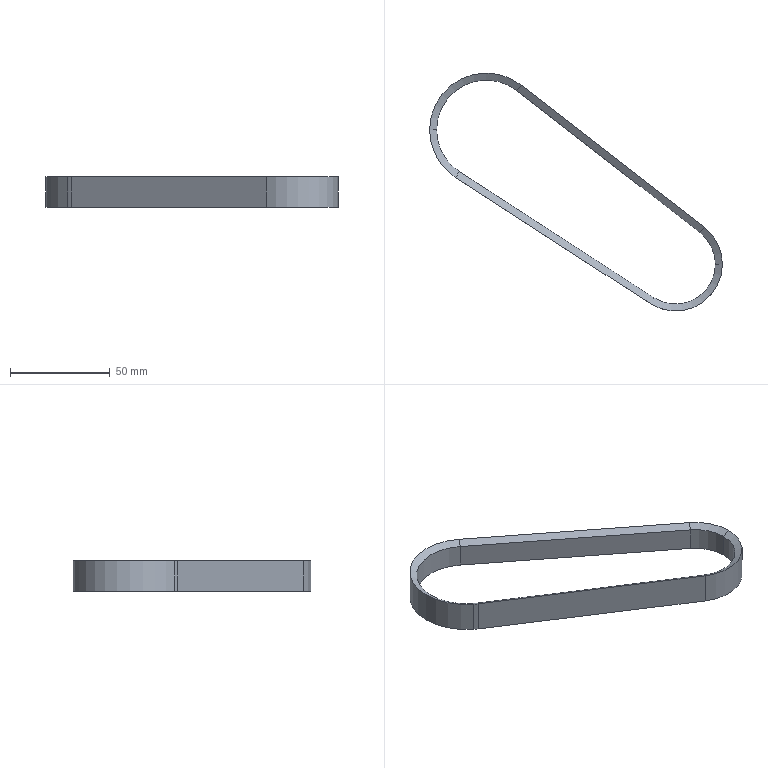Part | SolidWorks | features BaseBody 1 | 1 solid | 22 faces | box 147 x 119.5 x 15.423 mm | volume 18116 mm3 | cone 8 | plane 8 | cylinder 6 | commonest cylinder face diameters 40 x2 57 x2 47 x1 50 x1
STEP:
#1=CARTESIAN_POINT('',(-10.874,-16.786,2.021));
#2=VERTEX_POINT('',#1);
#3=CARTESIAN_POINT('',(20.,0.,2.021));
#4=VERTEX_POINT('',#3);
#5=CARTESIAN_POINT('',(0.,0.,2.021));
#6=DIRECTION('',(0.,0.,1.));
#7=DIRECTION('',(1.,0.,0.));
#8=AXIS2_PLACEMENT_3D('',#5,#6,#7);
#9=CIRCLE('',#8,20.);
#10=EDGE_CURVE('',#2,#4,#9,.T.);
#11=ORIENTED_EDGE('',*,*,#10,.T.);
#12=CARTESIAN_POINT('',(23.5,0.,0.));
#13=VERTEX_POINT('',#12);
#14=CARTESIAN_POINT('',(21.75,0.,1.01));
#15=DIRECTION('',(0.866,0.,-0.5001));
#16=VECTOR('',#15,1000.);
#17=LINE('',#14,#16);
#18=EDGE_CURVE('',#4,#13,#17,.T.);
#19=ORIENTED_EDGE('',*,*,#18,.T.);
#20=CARTESIAN_POINT('',(-12.777,-19.723,0.));
#21=VERTEX_POINT('',#20);
#22=CARTESIAN_POINT('',(0.,0.,0.));
#23=DIRECTION('',(0.,0.,-1.));
#24=DIRECTION('',(0.5437,0.8393,0.));
#25=AXIS2_PLACEMENT_3D('',#22,#23,#24);
#26=CIRCLE('',#25,23.5);
#27=EDGE_CURVE('',#13,#21,#26,.T.);
#28=ORIENTED_EDGE('',*,*,#27,.T.);
#29=CARTESIAN_POINT('',(-10.874,-16.786,2.021));
#30=DIRECTION('',(-0.4708,-0.7268,-0.5001));
#31=VECTOR('',#30,1000.);
#32=LINE('',#29,#31);
#33=EDGE_CURVE('',#2,#21,#32,.T.);
#34=ORIENTED_EDGE('',*,*,#33,.F.);
#35=EDGE_LOOP('',(#11,#19,#28,#34));
#36=FACE_OUTER_BOUND('',#35,.T.);
#37=CARTESIAN_POINT('',(0.,0.,1.01));
#38=DIRECTION('',(0.,0.,-1.));
#39=DIRECTION('',(1.,0.,0.));
#40=AXIS2_PLACEMENT_3D('',#37,#38,#39);
#41=CONICAL_SURFACE('',#40,21.75,1.047);
#42=ADVANCED_FACE('',(#36),#41,.F.);
#43=CARTESIAN_POINT('',(-79.659,87.239,2.021));
#44=VERTEX_POINT('',#43);
#45=CARTESIAN_POINT('',(-120.,67.5,2.021));
#46=VERTEX_POINT('',#45);
#47=CARTESIAN_POINT('',(-95.,67.5,2.021));
#48=DIRECTION('',(0.,0.,1.));
#49=DIRECTION('',(-1.,0.,0.));
#50=AXIS2_PLACEMENT_3D('',#47,#48,#49);
#51=CIRCLE('',#50,25.);
#52=EDGE_CURVE('',#44,#46,#51,.T.);
#53=ORIENTED_EDGE('',*,*,#52,.T.);
#54=CARTESIAN_POINT('',(-123.5,67.5,0.));
#55=VERTEX_POINT('',#54);
#56=CARTESIAN_POINT('',(-121.75,67.5,1.01));
#57=DIRECTION('',(-0.866,0.,-0.5001));
#58=VECTOR('',#57,1000.);
#59=LINE('',#56,#58);
#60=EDGE_CURVE('',#46,#55,#59,.T.);
#61=ORIENTED_EDGE('',*,*,#60,.T.);
#62=CARTESIAN_POINT('',(-77.511,90.003,0.));
#63=VERTEX_POINT('',#62);
#64=CARTESIAN_POINT('',(-95.,67.5,0.));
#65=DIRECTION('',(0.,0.,-1.));
#66=DIRECTION('',(-0.6136,-0.7896,0.));
#67=AXIS2_PLACEMENT_3D('',#64,#65,#66);
#68=CIRCLE('',#67,28.5);
#69=EDGE_CURVE('',#55,#63,#68,.T.);
#70=ORIENTED_EDGE('',*,*,#69,.T.);
#71=CARTESIAN_POINT('',(-79.659,87.239,2.021));
#72=DIRECTION('',(0.5314,0.6838,-0.5001));
#73=VECTOR('',#72,1000.);
#74=LINE('',#71,#73);
#75=EDGE_CURVE('',#44,#63,#74,.T.);
#76=ORIENTED_EDGE('',*,*,#75,.F.);
#77=EDGE_LOOP('',(#53,#61,#70,#76));
#78=FACE_OUTER_BOUND('',#77,.T.);
#79=CARTESIAN_POINT('',(-95.,67.5,1.01));
#80=DIRECTION('',(0.,0.,-1.));
#81=DIRECTION('',(-1.,0.,0.));
#82=AXIS2_PLACEMENT_3D('',#79,#80,#81);
#83=CONICAL_SURFACE('',#82,26.75,1.047);
#84=ADVANCED_FACE('',(#78),#83,.F.);
#85=CARTESIAN_POINT('',(20.,0.,13.402));
#86=VERTEX_POINT('',#85);
#87=CARTESIAN_POINT('',(-10.874,-16.786,13.402));
#88=VERTEX_POINT('',#87);
#89=CARTESIAN_POINT('',(0.,0.,13.402));
#90=DIRECTION('',(0.,0.,-1.));
#91=DIRECTION('',(1.,0.,0.));
#92=AXIS2_PLACEMENT_3D('',#89,#90,#91);
#93=CIRCLE('',#92,20.);
#94=EDGE_CURVE('',#86,#88,#93,.T.);
#95=ORIENTED_EDGE('',*,*,#94,.F.);
#96=CARTESIAN_POINT('',(20.,0.,0.));
#97=DIRECTION('',(0.,0.,-1.));
#98=VECTOR('',#97,1000.);
#99=LINE('',#96,#98);
#100=EDGE_CURVE('',#86,#4,#99,.T.);
#101=ORIENTED_EDGE('',*,*,#100,.T.);
#102=ORIENTED_EDGE('',*,*,#10,.F.);
#103=CARTESIAN_POINT('',(-10.874,-16.786,0.));
#104=DIRECTION('',(0.,0.,-1.));
#105=VECTOR('',#104,1000.);
#106=LINE('',#103,#105);
#107=EDGE_CURVE('',#88,#2,#106,.T.);
#108=ORIENTED_EDGE('',*,*,#107,.F.);
#109=EDGE_LOOP('',(#95,#101,#102,#108));
#110=FACE_OUTER_BOUND('',#109,.T.);
#111=CARTESIAN_POINT('',(0.,0.,0.));
#112=DIRECTION('',(0.,0.,-1.));
#113=DIRECTION('',(1.,0.,0.));
#114=AXIS2_PLACEMENT_3D('',#111,#112,#113);
#115=CYLINDRICAL_SURFACE('',#114,20.);
#116=ADVANCED_FACE('',(#110),#115,.F.);
#117=CARTESIAN_POINT('',(12.273,15.792,13.402));
#118=VERTEX_POINT('',#117);
#119=CARTESIAN_POINT('',(0.,0.,13.402));
#120=DIRECTION('',(0.,0.,-1.));
#121=DIRECTION('',(1.,0.,0.));
#122=AXIS2_PLACEMENT_3D('',#119,#120,#121);
#123=CIRCLE('',#122,20.);
#124=EDGE_CURVE('',#118,#86,#123,.T.);
#125=ORIENTED_EDGE('',*,*,#124,.T.);
#126=CARTESIAN_POINT('',(23.5,0.,15.423));
#127=VERTEX_POINT('',#126);
#128=CARTESIAN_POINT('',(21.75,0.,14.412));
#129=DIRECTION('',(0.866,0.,0.5001));
#130=VECTOR('',#129,1000.);
#131=LINE('',#128,#130);
#132=EDGE_CURVE('',#86,#127,#131,.T.);
#133=ORIENTED_EDGE('',*,*,#132,.T.);
#134=CARTESIAN_POINT('',(14.421,18.555,15.423));
#135=VERTEX_POINT('',#134);
#136=CARTESIAN_POINT('',(0.,0.,15.423));
#137=DIRECTION('',(0.,0.,1.));
#138=DIRECTION('',(0.5437,0.8393,0.));
#139=AXIS2_PLACEMENT_3D('',#136,#137,#138);
#140=CIRCLE('',#139,23.5);
#141=EDGE_CURVE('',#127,#135,#140,.T.);
#142=ORIENTED_EDGE('',*,*,#141,.T.);
#143=CARTESIAN_POINT('',(14.421,18.555,15.423));
#144=DIRECTION('',(-0.5314,-0.6838,-0.5001));
#145=VECTOR('',#144,1000.);
#146=LINE('',#143,#145);
#147=EDGE_CURVE('',#135,#118,#146,.T.);
#148=ORIENTED_EDGE('',*,*,#147,.T.);
#149=EDGE_LOOP('',(#125,#133,#142,#148));
#150=FACE_OUTER_BOUND('',#149,.T.);
#151=CARTESIAN_POINT('',(0.,0.,14.412));
#152=DIRECTION('',(0.,0.,1.));
#153=DIRECTION('',(1.,0.,0.));
#154=AXIS2_PLACEMENT_3D('',#151,#152,#153);
#155=CONICAL_SURFACE('',#154,21.75,1.047);
#156=ADVANCED_FACE('',(#150),#155,.F.);
#157=CARTESIAN_POINT('',(-108.592,46.518,13.402));
#158=VERTEX_POINT('',#157);
#159=CARTESIAN_POINT('',(-120.,67.5,13.402));
#160=VERTEX_POINT('',#159);
#161=CARTESIAN_POINT('',(-95.,67.5,13.402));
#162=DIRECTION('',(0.,0.,-1.));
#163=DIRECTION('',(-1.,0.,0.));
#164=AXIS2_PLACEMENT_3D('',#161,#162,#163);
#165=CIRCLE('',#164,25.);
#166=EDGE_CURVE('',#158,#160,#165,.T.);
#167=ORIENTED_EDGE('',*,*,#166,.T.);
#168=CARTESIAN_POINT('',(-123.5,67.5,15.423));
#169=VERTEX_POINT('',#168);
#170=CARTESIAN_POINT('',(-121.75,67.5,14.412));
#171=DIRECTION('',(-0.866,0.,0.5001));
#172=VECTOR('',#171,1000.);
#173=LINE('',#170,#172);
#174=EDGE_CURVE('',#160,#169,#173,.T.);
#175=ORIENTED_EDGE('',*,*,#174,.T.);
#176=CARTESIAN_POINT('',(-112.489,44.997,15.423));
#177=VERTEX_POINT('',#176);
#178=CARTESIAN_POINT('',(-95.,67.5,15.423));
#179=DIRECTION('',(0.,0.,1.));
#180=DIRECTION('',(-0.6136,-0.7896,0.));
#181=AXIS2_PLACEMENT_3D('',#178,#179,#180);
#182=CIRCLE('',#181,28.5);
#183=EDGE_CURVE('',#169,#177,#182,.T.);
#184=ORIENTED_EDGE('',*,*,#183,.T.);
#185=CARTESIAN_POINT('',(-110.495,43.581,15.423));
#186=VERTEX_POINT('',#185);
#187=CARTESIAN_POINT('',(-95.,67.5,15.423));
#188=DIRECTION('',(0.,0.,1.));
#189=DIRECTION('',(-0.6136,-0.7896,0.));
#190=AXIS2_PLACEMENT_3D('',#187,#188,#189);
#191=CIRCLE('',#190,28.5);
#192=EDGE_CURVE('',#177,#186,#191,.T.);
#193=ORIENTED_EDGE('',*,*,#192,.T.);
#194=CARTESIAN_POINT('',(-108.592,46.518,13.402));
#195=DIRECTION('',(-0.4708,-0.7268,0.5001));
#196=VECTOR('',#195,1000.);
#197=LINE('',#194,#196);
#198=EDGE_CURVE('',#158,#186,#197,.T.);
#199=ORIENTED_EDGE('',*,*,#198,.F.);
#200=EDGE_LOOP('',(#167,#175,#184,#193,#199));
#201=FACE_OUTER_BOUND('',#200,.T.);
#202=CARTESIAN_POINT('',(-95.,67.5,14.412));
#203=DIRECTION('',(0.,0.,1.));
#204=DIRECTION('',(-1.,0.,0.));
#205=AXIS2_PLACEMENT_3D('',#202,#203,#204);
#206=CONICAL_SURFACE('',#205,26.75,1.047);
#207=ADVANCED_FACE('',(#201),#206,.F.);
#208=ORIENTED_EDGE('',*,*,#192,.F.);
#209=CARTESIAN_POINT('',(-112.489,44.997,0.));
#210=VERTEX_POINT('',#209);
#211=CARTESIAN_POINT('',(-112.489,44.997,0.));
#212=DIRECTION('',(0.,0.,-1.));
#213=VECTOR('',#212,1000.);
#214=LINE('',#211,#213);
#215=EDGE_CURVE('',#177,#210,#214,.T.);
#216=ORIENTED_EDGE('',*,*,#215,.T.);
#217=CARTESIAN_POINT('',(-110.495,43.581,0.));
#218=VERTEX_POINT('',#217);
#219=CARTESIAN_POINT('',(-95.,67.5,0.));
#220=DIRECTION('',(0.,0.,-1.));
#221=DIRECTION('',(-0.6136,-0.7896,0.));
#222=AXIS2_PLACEMENT_3D('',#219,#220,#221);
#223=CIRCLE('',#222,28.5);
#224=EDGE_CURVE('',#218,#210,#223,.T.);
#225=ORIENTED_EDGE('',*,*,#224,.F.);
#226=CARTESIAN_POINT('',(-110.495,43.581,0.));
#227=DIRECTION('',(0.,0.,1.));
#228=VECTOR('',#227,1000.);
#229=LINE('',#226,#228);
#230=EDGE_CURVE('',#218,#186,#229,.T.);
#231=ORIENTED_EDGE('',*,*,#230,.T.);
#232=EDGE_LOOP('',(#208,#216,#225,#231));
#233=FACE_OUTER_BOUND('',#232,.T.);
#234=CARTESIAN_POINT('',(-95.,67.5,0.));
#235=DIRECTION('',(0.,0.,-1.));
#236=DIRECTION('',(-0.6136,-0.7896,0.));
#237=AXIS2_PLACEMENT_3D('',#234,#235,#236);
#238=CYLINDRICAL_SURFACE('',#237,28.5);
#239=ADVANCED_FACE('',(#233),#238,.T.);
#240=ORIENTED_EDGE('',*,*,#33,.T.);
#241=CARTESIAN_POINT('',(-12.777,-19.723,0.));
#242=DIRECTION('',(-0.8393,0.5437,0.));
#243=VECTOR('',#242,1000.);
#244=LINE('',#241,#243);
#245=EDGE_CURVE('',#21,#218,#244,.T.);
#246=ORIENTED_EDGE('',*,*,#245,.T.);
#247=CARTESIAN_POINT('',(-108.592,46.518,2.021));
#248=VERTEX_POINT('',#247);
#249=CARTESIAN_POINT('',(-110.495,43.581,0.));
#250=DIRECTION('',(0.4708,0.7268,0.5001));
#251=VECTOR('',#250,1000.);
#252=LINE('',#249,#251);
#253=EDGE_CURVE('',#218,#248,#252,.T.);
#254=ORIENTED_EDGE('',*,*,#253,.T.);
#255=CARTESIAN_POINT('',(-85.355,31.464,2.021));
#256=DIRECTION('',(0.8393,-0.5437,0.));
#257=VECTOR('',#256,1000.);
#258=LINE('',#255,#257);
#259=EDGE_CURVE('',#248,#2,#258,.T.);
#260=ORIENTED_EDGE('',*,*,#259,.T.);
#261=EDGE_LOOP('',(#240,#246,#254,#260));
#262=FACE_OUTER_BOUND('',#261,.T.);
#263=CARTESIAN_POINT('',(-86.306,29.996,1.01));
#264=DIRECTION('',(0.2719,0.4197,-0.866));
#265=DIRECTION('',(-0.9541,0.,-0.2995));
#266=AXIS2_PLACEMENT_3D('',#263,#264,#265);
#267=PLANE('',#266);
#268=ADVANCED_FACE('',(#262),#267,.T.);
#269=ORIENTED_EDGE('',*,*,#75,.T.);
#270=CARTESIAN_POINT('',(14.421,18.555,0.));
#271=VERTEX_POINT('',#270);
#272=CARTESIAN_POINT('',(-77.511,90.003,0.));
#273=DIRECTION('',(0.7896,-0.6136,0.));
#274=VECTOR('',#273,1000.);
#275=LINE('',#272,#274);
#276=EDGE_CURVE('',#63,#271,#275,.T.);
#277=ORIENTED_EDGE('',*,*,#276,.T.);
#278=CARTESIAN_POINT('',(12.273,15.792,2.021));
#279=VERTEX_POINT('',#278);
#280=CARTESIAN_POINT('',(12.273,15.792,2.021));
#281=DIRECTION('',(0.5314,0.6838,-0.5001));
#282=VECTOR('',#281,1000.);
#283=LINE('',#280,#282);
#284=EDGE_CURVE('',#279,#271,#283,.T.);
#285=ORIENTED_EDGE('',*,*,#284,.F.);
#286=CARTESIAN_POINT('',(-11.831,34.525,2.021));
#287=DIRECTION('',(-0.7896,0.6136,0.));
#288=VECTOR('',#287,1000.);
#289=LINE('',#286,#288);
#290=EDGE_CURVE('',#279,#44,#289,.T.);
#291=ORIENTED_EDGE('',*,*,#290,.T.);
#292=EDGE_LOOP('',(#269,#277,#285,#291));
#293=FACE_OUTER_BOUND('',#292,.T.);
#294=CARTESIAN_POINT('',(-10.758,35.907,1.01));
#295=DIRECTION('',(-0.3069,-0.3948,-0.866));
#296=DIRECTION('',(0.,-0.9099,0.4148));
#297=AXIS2_PLACEMENT_3D('',#294,#295,#296);
#298=PLANE('',#297);
#299=ADVANCED_FACE('',(#293),#298,.T.);
#300=ORIENTED_EDGE('',*,*,#259,.F.);
#301=CARTESIAN_POINT('',(-108.592,46.518,0.));
#302=DIRECTION('',(0.,0.,-1.));
#303=VECTOR('',#302,1000.);
#304=LINE('',#301,#303);
#305=EDGE_CURVE('',#158,#248,#304,.T.);
#306=ORIENTED_EDGE('',*,*,#305,.F.);
#307=CARTESIAN_POINT('',(-85.355,31.464,13.402));
#308=DIRECTION('',(-0.8393,0.5437,0.));
#309=VECTOR('',#308,1000.);
#310=LINE('',#307,#309);
#311=EDGE_CURVE('',#88,#158,#310,.T.);
#312=ORIENTED_EDGE('',*,*,#311,.F.);
#313=ORIENTED_EDGE('',*,*,#107,.T.);
#314=EDGE_LOOP('',(#300,#306,#312,#313));
#315=FACE_OUTER_BOUND('',#314,.T.);
#316=CARTESIAN_POINT('',(-108.592,46.518,0.));
#317=DIRECTION('',(-0.5437,-0.8393,0.));
#318=DIRECTION('',(-0.8393,0.5437,0.));
#319=AXIS2_PLACEMENT_3D('',#316,#317,#318);
#320=PLANE('',#319);
#321=ADVANCED_FACE('',(#315),#320,.F.);
#322=ORIENTED_EDGE('',*,*,#198,.T.);
#323=CARTESIAN_POINT('',(-12.777,-19.723,15.423));
#324=VERTEX_POINT('',#323);
#325=CARTESIAN_POINT('',(-12.777,-19.723,15.423));
#326=DIRECTION('',(0.8393,-0.5437,0.));
#327=VECTOR('',#326,1000.);
#328=LINE('',#325,#327);
#329=EDGE_CURVE('',#186,#324,#328,.T.);
#330=ORIENTED_EDGE('',*,*,#329,.T.);
#331=CARTESIAN_POINT('',(-10.874,-16.786,13.402));
#332=DIRECTION('',(-0.4708,-0.7268,0.5001));
#333=VECTOR('',#332,1000.);
#334=LINE('',#331,#333);
#335=EDGE_CURVE('',#88,#324,#334,.T.);
#336=ORIENTED_EDGE('',*,*,#335,.F.);
#337=ORIENTED_EDGE('',*,*,#311,.T.);
#338=EDGE_LOOP('',(#322,#330,#336,#337));
#339=FACE_OUTER_BOUND('',#338,.T.);
#340=CARTESIAN_POINT('',(-86.306,29.996,14.412));
#341=DIRECTION('',(0.2719,0.4197,0.866));
#342=DIRECTION('',(0.8393,-0.5437,0.));
#343=AXIS2_PLACEMENT_3D('',#340,#341,#342);
#344=PLANE('',#343);
#345=ADVANCED_FACE('',(#339),#344,.T.);
#346=ORIENTED_EDGE('',*,*,#147,.F.);
#347=CARTESIAN_POINT('',(-77.511,90.003,15.423));
#348=VERTEX_POINT('',#347);
#349=CARTESIAN_POINT('',(-77.511,90.003,15.423));
#350=DIRECTION('',(-0.7896,0.6136,0.));
#351=VECTOR('',#350,1000.);
#352=LINE('',#349,#351);
#353=EDGE_CURVE('',#135,#348,#352,.T.);
#354=ORIENTED_EDGE('',*,*,#353,.T.);
#355=CARTESIAN_POINT('',(-79.659,87.239,13.402));
#356=VERTEX_POINT('',#355);
#357=CARTESIAN_POINT('',(-79.659,87.239,13.402));
#358=DIRECTION('',(0.5314,0.6838,0.5001));
#359=VECTOR('',#358,1000.);
#360=LINE('',#357,#359);
#361=EDGE_CURVE('',#356,#348,#360,.T.);
#362=ORIENTED_EDGE('',*,*,#361,.F.);
#363=CARTESIAN_POINT('',(-11.831,34.525,13.402));
#364=DIRECTION('',(0.7896,-0.6136,0.));
#365=VECTOR('',#364,1000.);
#366=LINE('',#363,#365);
#367=EDGE_CURVE('',#356,#118,#366,.T.);
#368=ORIENTED_EDGE('',*,*,#367,.T.);
#369=EDGE_LOOP('',(#346,#354,#362,#368));
#370=FACE_OUTER_BOUND('',#369,.T.);
#371=CARTESIAN_POINT('',(-10.758,35.907,14.412));
#372=DIRECTION('',(-0.3069,-0.3948,0.866));
#373=DIRECTION('',(-0.7896,0.6136,0.));
#374=AXIS2_PLACEMENT_3D('',#371,#372,#373);
#375=PLANE('',#374);
#376=ADVANCED_FACE('',(#370),#375,.T.);
#377=ORIENTED_EDGE('',*,*,#290,.F.);
#378=CARTESIAN_POINT('',(12.273,15.792,0.));
#379=DIRECTION('',(0.,0.,-1.));
#380=VECTOR('',#379,1000.);
#381=LINE('',#378,#380);
#382=EDGE_CURVE('',#118,#279,#381,.T.);
#383=ORIENTED_EDGE('',*,*,#382,.F.);
#384=ORIENTED_EDGE('',*,*,#367,.F.);
#385=CARTESIAN_POINT('',(-79.659,87.239,0.));
#386=DIRECTION('',(0.,0.,-1.));
#387=VECTOR('',#386,1000.);
#388=LINE('',#385,#387);
#389=EDGE_CURVE('',#356,#44,#388,.T.);
#390=ORIENTED_EDGE('',*,*,#389,.T.);
#391=EDGE_LOOP('',(#377,#383,#384,#390));
#392=FACE_OUTER_BOUND('',#391,.T.);
#393=CARTESIAN_POINT('',(12.273,15.792,0.));
#394=DIRECTION('',(0.6136,0.7896,0.));
#395=DIRECTION('',(0.,0.,-1.));
#396=AXIS2_PLACEMENT_3D('',#393,#394,#395);
#397=PLANE('',#396);
#398=ADVANCED_FACE('',(#392),#397,.F.);
#399=ORIENTED_EDGE('',*,*,#52,.F.);
#400=ORIENTED_EDGE('',*,*,#389,.F.);
#401=CARTESIAN_POINT('',(-95.,67.5,13.402));
#402=DIRECTION('',(0.,0.,-1.));
#403=DIRECTION('',(-1.,0.,0.));
#404=AXIS2_PLACEMENT_3D('',#401,#402,#403);
#405=CIRCLE('',#404,25.);
#406=EDGE_CURVE('',#160,#356,#405,.T.);
#407=ORIENTED_EDGE('',*,*,#406,.F.);
#408=ORIENTED_EDGE('',*,*,#166,.F.);
#409=ORIENTED_EDGE('',*,*,#305,.T.);
#410=CARTESIAN_POINT('',(-95.,67.5,2.021));
#411=DIRECTION('',(0.,0.,1.));
#412=DIRECTION('',(-1.,0.,0.));
#413=AXIS2_PLACEMENT_3D('',#410,#411,#412);
#414=CIRCLE('',#413,25.);
#415=EDGE_CURVE('',#46,#248,#414,.T.);
#416=ORIENTED_EDGE('',*,*,#415,.F.);
#417=EDGE_LOOP('',(#399,#400,#407,#408,#409,#416));
#418=FACE_OUTER_BOUND('',#417,.T.);
#419=CARTESIAN_POINT('',(-95.,67.5,0.));
#420=DIRECTION('',(0.,0.,-1.));
#421=DIRECTION('',(1.,0.,0.));
#422=AXIS2_PLACEMENT_3D('',#419,#420,#421);
#423=CYLINDRICAL_SURFACE('',#422,25.);
#424=ADVANCED_FACE('',(#418),#423,.F.);
#425=CARTESIAN_POINT('',(0.,0.,0.));
#426=DIRECTION('',(0.,0.,-1.));
#427=DIRECTION('',(0.5437,0.8393,0.));
#428=AXIS2_PLACEMENT_3D('',#425,#426,#427);
#429=CIRCLE('',#428,23.5);
#430=EDGE_CURVE('',#271,#13,#429,.T.);
#431=ORIENTED_EDGE('',*,*,#430,.F.);
#432=CARTESIAN_POINT('',(14.421,18.555,0.));
#433=DIRECTION('',(0.,0.,1.));
#434=VECTOR('',#433,1000.);
#435=LINE('',#432,#434);
#436=EDGE_CURVE('',#271,#135,#435,.T.);
#437=ORIENTED_EDGE('',*,*,#436,.T.);
#438=ORIENTED_EDGE('',*,*,#141,.F.);
#439=CARTESIAN_POINT('',(0.,0.,15.423));
#440=DIRECTION('',(0.,0.,1.));
#441=DIRECTION('',(0.5437,0.8393,0.));
#442=AXIS2_PLACEMENT_3D('',#439,#440,#441);
#443=CIRCLE('',#442,23.5);
#444=EDGE_CURVE('',#324,#127,#443,.T.);
#445=ORIENTED_EDGE('',*,*,#444,.F.);
#446=CARTESIAN_POINT('',(-12.777,-19.723,0.));
#447=DIRECTION('',(0.,0.,1.));
#448=VECTOR('',#447,1000.);
#449=LINE('',#446,#448);
#450=EDGE_CURVE('',#21,#324,#449,.T.);
#451=ORIENTED_EDGE('',*,*,#450,.F.);
#452=ORIENTED_EDGE('',*,*,#27,.F.);
#453=EDGE_LOOP('',(#431,#437,#438,#445,#451,#452));
#454=FACE_OUTER_BOUND('',#453,.T.);
#455=CARTESIAN_POINT('',(0.,0.,0.));
#456=DIRECTION('',(0.,0.,-1.));
#457=DIRECTION('',(0.5437,0.8393,0.));
#458=AXIS2_PLACEMENT_3D('',#455,#456,#457);
#459=CYLINDRICAL_SURFACE('',#458,23.5);
#460=ADVANCED_FACE('',(#454),#459,.T.);
#461=ORIENTED_EDGE('',*,*,#245,.F.);
#462=ORIENTED_EDGE('',*,*,#450,.T.);
#463=ORIENTED_EDGE('',*,*,#329,.F.);
#464=ORIENTED_EDGE('',*,*,#230,.F.);
#465=EDGE_LOOP('',(#461,#462,#463,#464));
#466=FACE_OUTER_BOUND('',#465,.T.);
#467=CARTESIAN_POINT('',(-110.495,43.581,0.));
#468=DIRECTION('',(-0.5437,-0.8393,0.));
#469=DIRECTION('',(-0.8393,0.5437,0.));
#470=AXIS2_PLACEMENT_3D('',#467,#468,#469);
#471=PLANE('',#470);
#472=ADVANCED_FACE('',(#466),#471,.T.);
#473=ORIENTED_EDGE('',*,*,#276,.F.);
#474=CARTESIAN_POINT('',(-77.511,90.003,0.));
#475=DIRECTION('',(0.,0.,1.));
#476=VECTOR('',#475,1000.);
#477=LINE('',#474,#476);
#478=EDGE_CURVE('',#63,#348,#477,.T.);
#479=ORIENTED_EDGE('',*,*,#478,.T.);
#480=ORIENTED_EDGE('',*,*,#353,.F.);
#481=ORIENTED_EDGE('',*,*,#436,.F.);
#482=EDGE_LOOP('',(#473,#479,#480,#481));
#483=FACE_OUTER_BOUND('',#482,.T.);
#484=CARTESIAN_POINT('',(14.421,18.555,0.));
#485=DIRECTION('',(0.6136,0.7896,0.));
#486=DIRECTION('',(0.,0.,-1.));
#487=AXIS2_PLACEMENT_3D('',#484,#485,#486);
#488=PLANE('',#487);
#489=ADVANCED_FACE('',(#483),#488,.T.);
#490=ORIENTED_EDGE('',*,*,#215,.F.);
#491=ORIENTED_EDGE('',*,*,#183,.F.);
#492=CARTESIAN_POINT('',(-95.,67.5,15.423));
#493=DIRECTION('',(0.,0.,1.));
#494=DIRECTION('',(-0.6136,-0.7896,0.));
#495=AXIS2_PLACEMENT_3D('',#492,#493,#494);
#496=CIRCLE('',#495,28.5);
#497=EDGE_CURVE('',#348,#169,#496,.T.);
#498=ORIENTED_EDGE('',*,*,#497,.F.);
#499=ORIENTED_EDGE('',*,*,#478,.F.);
#500=ORIENTED_EDGE('',*,*,#69,.F.);
#501=CARTESIAN_POINT('',(-95.,67.5,0.));
#502=DIRECTION('',(0.,0.,-1.));
#503=DIRECTION('',(-0.6136,-0.7896,0.));
#504=AXIS2_PLACEMENT_3D('',#501,#502,#503);
#505=CIRCLE('',#504,28.5);
#506=EDGE_CURVE('',#210,#55,#505,.T.);
#507=ORIENTED_EDGE('',*,*,#506,.F.);
#508=EDGE_LOOP('',(#490,#491,#498,#499,#500,#507));
#509=FACE_OUTER_BOUND('',#508,.T.);
#510=CARTESIAN_POINT('',(-95.,67.5,0.));
#511=DIRECTION('',(0.,0.,-1.));
#512=DIRECTION('',(-0.6136,-0.7896,0.));
#513=AXIS2_PLACEMENT_3D('',#510,#511,#512);
#514=CYLINDRICAL_SURFACE('',#513,28.5);
#515=ADVANCED_FACE('',(#509),#514,.T.);
#516=ORIENTED_EDGE('',*,*,#174,.F.);
#517=ORIENTED_EDGE('',*,*,#406,.T.);
#518=ORIENTED_EDGE('',*,*,#361,.T.);
#519=ORIENTED_EDGE('',*,*,#497,.T.);
#520=EDGE_LOOP('',(#516,#517,#518,#519));
#521=FACE_OUTER_BOUND('',#520,.T.);
#522=CARTESIAN_POINT('',(-95.,67.5,14.412));
#523=DIRECTION('',(0.,0.,1.));
#524=DIRECTION('',(-1.,0.,0.));
#525=AXIS2_PLACEMENT_3D('',#522,#523,#524);
#526=CONICAL_SURFACE('',#525,26.75,1.047);
#527=ADVANCED_FACE('',(#521),#526,.F.);
#528=ORIENTED_EDGE('',*,*,#132,.F.);
#529=ORIENTED_EDGE('',*,*,#94,.T.);
#530=ORIENTED_EDGE('',*,*,#335,.T.);
#531=ORIENTED_EDGE('',*,*,#444,.T.);
#532=EDGE_LOOP('',(#528,#529,#530,#531));
#533=FACE_OUTER_BOUND('',#532,.T.);
#534=CARTESIAN_POINT('',(0.,0.,14.412));
#535=DIRECTION('',(0.,0.,1.));
#536=DIRECTION('',(1.,0.,0.));
#537=AXIS2_PLACEMENT_3D('',#534,#535,#536);
#538=CONICAL_SURFACE('',#537,21.75,1.047);
#539=ADVANCED_FACE('',(#533),#538,.F.);
#540=ORIENTED_EDGE('',*,*,#100,.F.);
#541=ORIENTED_EDGE('',*,*,#124,.F.);
#542=ORIENTED_EDGE('',*,*,#382,.T.);
#543=CARTESIAN_POINT('',(0.,0.,2.021));
#544=DIRECTION('',(0.,0.,1.));
#545=DIRECTION('',(1.,0.,0.));
#546=AXIS2_PLACEMENT_3D('',#543,#544,#545);
#547=CIRCLE('',#546,20.);
#548=EDGE_CURVE('',#4,#279,#547,.T.);
#549=ORIENTED_EDGE('',*,*,#548,.F.);
#550=EDGE_LOOP('',(#540,#541,#542,#549));
#551=FACE_OUTER_BOUND('',#550,.T.);
#552=CARTESIAN_POINT('',(0.,0.,0.));
#553=DIRECTION('',(0.,0.,-1.));
#554=DIRECTION('',(1.,0.,0.));
#555=AXIS2_PLACEMENT_3D('',#552,#553,#554);
#556=CYLINDRICAL_SURFACE('',#555,20.);
#557=ADVANCED_FACE('',(#551),#556,.F.);
#558=ORIENTED_EDGE('',*,*,#60,.F.);
#559=ORIENTED_EDGE('',*,*,#415,.T.);
#560=ORIENTED_EDGE('',*,*,#253,.F.);
#561=ORIENTED_EDGE('',*,*,#224,.T.);
#562=ORIENTED_EDGE('',*,*,#506,.T.);
#563=EDGE_LOOP('',(#558,#559,#560,#561,#562));
#564=FACE_OUTER_BOUND('',#563,.T.);
#565=CARTESIAN_POINT('',(-95.,67.5,1.01));
#566=DIRECTION('',(0.,0.,-1.));
#567=DIRECTION('',(-1.,0.,0.));
#568=AXIS2_PLACEMENT_3D('',#565,#566,#567);
#569=CONICAL_SURFACE('',#568,26.75,1.047);
#570=ADVANCED_FACE('',(#564),#569,.F.);
#571=ORIENTED_EDGE('',*,*,#18,.F.);
#572=ORIENTED_EDGE('',*,*,#548,.T.);
#573=ORIENTED_EDGE('',*,*,#284,.T.);
#574=ORIENTED_EDGE('',*,*,#430,.T.);
#575=EDGE_LOOP('',(#571,#572,#573,#574));
#576=FACE_OUTER_BOUND('',#575,.T.);
#577=CARTESIAN_POINT('',(0.,0.,1.01));
#578=DIRECTION('',(0.,0.,-1.));
#579=DIRECTION('',(1.,0.,0.));
#580=AXIS2_PLACEMENT_3D('',#577,#578,#579);
#581=CONICAL_SURFACE('',#580,21.75,1.047);
#582=ADVANCED_FACE('',(#576),#581,.F.);
#583=CLOSED_SHELL('',(#42,#84,#116,#156,#207,#239,#268,#299,#321,#345,#376,#398,#424,#460,#472,#489,#515,#527,#539,#557,#570,#582));
#584=MANIFOLD_SOLID_BREP('',#583);
#585=CARTESIAN_POINT('',(0.,0.,0.));
#586=DIRECTION('',(0.,0.,1.));
#587=DIRECTION('',(1.,0.,0.));
#588=AXIS2_PLACEMENT_3D('',#585,#586,#587);
#589=(LENGTH_UNIT()NAMED_UNIT(*)SI_UNIT(.MILLI.,.METRE.));
#590=UNCERTAINTY_MEASURE_WITH_UNIT(LENGTH_MEASURE(0.00001),#589,'','');
#591=(NAMED_UNIT(*)PLANE_ANGLE_UNIT()SI_UNIT($,.RADIAN.));
#592=(NAMED_UNIT(*)SI_UNIT($,.STERADIAN.)SOLID_ANGLE_UNIT());
#593=(GEOMETRIC_REPRESENTATION_CONTEXT(3)GLOBAL_UNCERTAINTY_ASSIGNED_CONTEXT((#590))GLOBAL_UNIT_ASSIGNED_CONTEXT((#589,#591,#592))REPRESENTATION_CONTEXT('',''));
#594=ADVANCED_BREP_SHAPE_REPRESENTATION('',(#584,#588),#593);